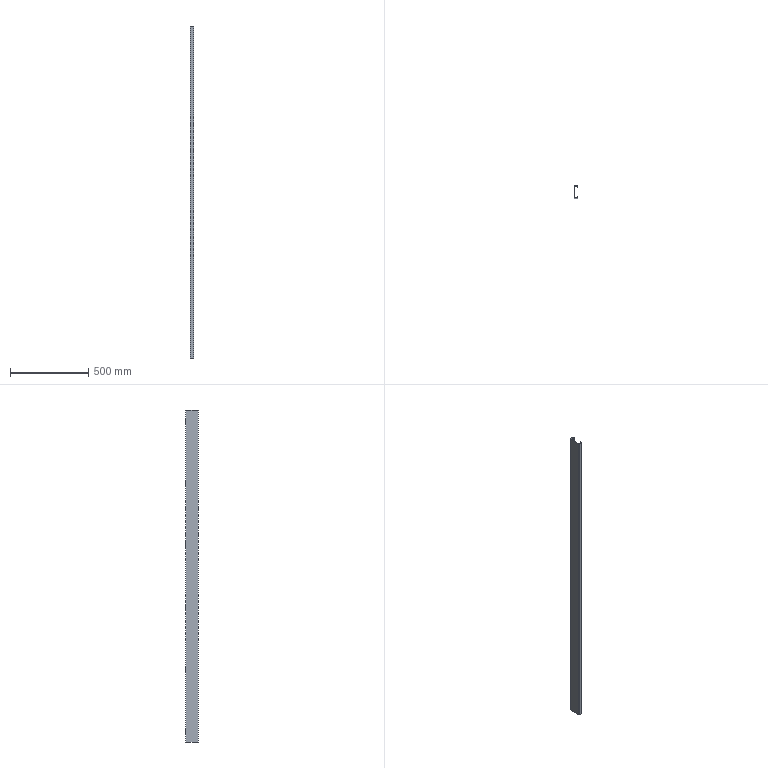Part | SolidWorks | features ICE 7, Cut 3, EdgeFlange 2, MirrorPattern 2, Fillet 1, FlatPattern 1, SMBaseFlange 1, SheetMetal 1 | 1 solid | 96 faces | box 25 x 80 x 2116 mm | volume 374202 mm3 | cylinder 54 | plane 42 | commonest cylinder face diameters 6.2 x28 9 x18 1 x4 3.4 x4